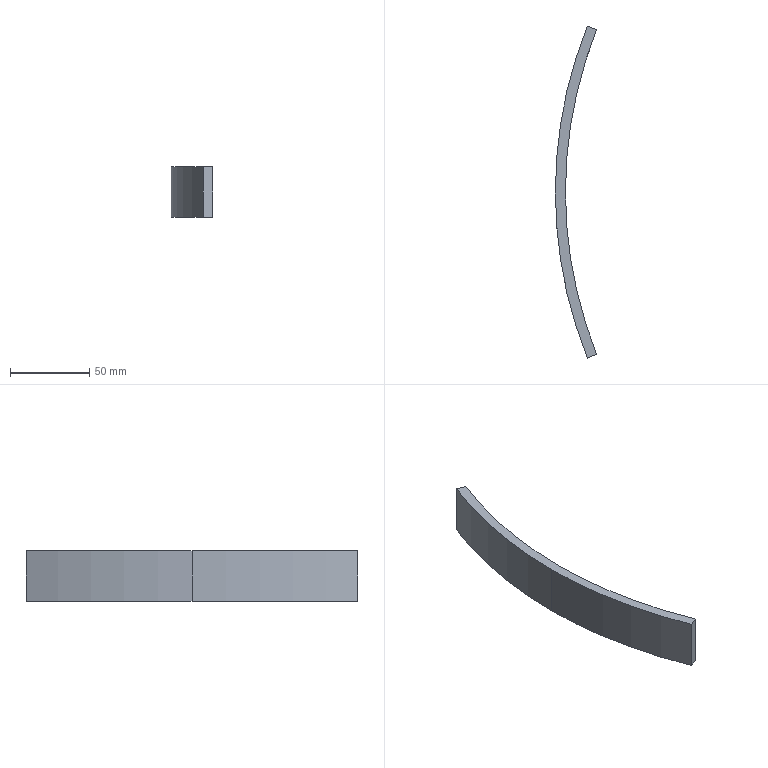Part | SolidWorks | features Extrusion 1 | 1 solid | 8 faces | box 25.986 x 209.322 x 31.75 mm | volume 42745 mm3 | cylinder 4 | plane 4 | commonest cylinder face diameters 552.7 x2 565.4 x2
STEP:
#1=CARTESIAN_POINT('',(-282.7,0.,31.75));
#2=VERTEX_POINT('',#1);
#3=CARTESIAN_POINT('',(-262.613,-104.661,31.75));
#4=VERTEX_POINT('',#3);
#5=CARTESIAN_POINT('',(0.,0.,31.75));
#6=DIRECTION('',(0.,0.,1.));
#7=DIRECTION('',(1.,0.,0.));
#8=AXIS2_PLACEMENT_3D('',#5,#6,#7);
#9=CIRCLE('',#8,282.7);
#10=EDGE_CURVE('',#2,#4,#9,.T.);
#11=ORIENTED_EDGE('',*,*,#10,.F.);
#12=CARTESIAN_POINT('',(-282.7,0.,0.));
#13=VERTEX_POINT('',#12);
#14=CARTESIAN_POINT('',(-282.7,0.,31.75));
#15=DIRECTION('',(0.,0.,-1.));
#16=VECTOR('',#15,1000.);
#17=LINE('',#14,#16);
#18=EDGE_CURVE('',#2,#13,#17,.T.);
#19=ORIENTED_EDGE('',*,*,#18,.T.);
#20=CARTESIAN_POINT('',(-262.613,-104.661,0.));
#21=VERTEX_POINT('',#20);
#22=CARTESIAN_POINT('',(0.,0.,0.));
#23=DIRECTION('',(0.,0.,1.));
#24=DIRECTION('',(1.,0.,0.));
#25=AXIS2_PLACEMENT_3D('',#22,#23,#24);
#26=CIRCLE('',#25,282.7);
#27=EDGE_CURVE('',#13,#21,#26,.T.);
#28=ORIENTED_EDGE('',*,*,#27,.T.);
#29=CARTESIAN_POINT('',(-262.613,-104.661,31.75));
#30=DIRECTION('',(0.,0.,-1.));
#31=VECTOR('',#30,1000.);
#32=LINE('',#29,#31);
#33=EDGE_CURVE('',#4,#21,#32,.T.);
#34=ORIENTED_EDGE('',*,*,#33,.F.);
#35=EDGE_LOOP('',(#11,#19,#28,#34));
#36=FACE_OUTER_BOUND('',#35,.T.);
#37=CARTESIAN_POINT('',(0.,0.,31.75));
#38=DIRECTION('',(0.,0.,-1.));
#39=DIRECTION('',(-1.,0.,0.));
#40=AXIS2_PLACEMENT_3D('',#37,#38,#39);
#41=CYLINDRICAL_SURFACE('',#40,282.7);
#42=ADVANCED_FACE('',(#36),#41,.T.);
#43=CARTESIAN_POINT('',(-276.35,0.,31.75));
#44=VERTEX_POINT('',#43);
#45=CARTESIAN_POINT('',(-256.714,102.31,31.75));
#46=VERTEX_POINT('',#45);
#47=CARTESIAN_POINT('',(0.,0.,31.75));
#48=DIRECTION('',(0.,0.,-1.));
#49=DIRECTION('',(1.,0.,0.));
#50=AXIS2_PLACEMENT_3D('',#47,#48,#49);
#51=CIRCLE('',#50,276.35);
#52=EDGE_CURVE('',#44,#46,#51,.T.);
#53=ORIENTED_EDGE('',*,*,#52,.F.);
#54=CARTESIAN_POINT('',(-276.35,0.,0.));
#55=VERTEX_POINT('',#54);
#56=CARTESIAN_POINT('',(-276.35,0.,31.75));
#57=DIRECTION('',(0.,0.,-1.));
#58=VECTOR('',#57,1000.);
#59=LINE('',#56,#58);
#60=EDGE_CURVE('',#44,#55,#59,.T.);
#61=ORIENTED_EDGE('',*,*,#60,.T.);
#62=CARTESIAN_POINT('',(-256.714,102.31,0.));
#63=VERTEX_POINT('',#62);
#64=CARTESIAN_POINT('',(0.,0.,0.));
#65=DIRECTION('',(0.,0.,-1.));
#66=DIRECTION('',(1.,0.,0.));
#67=AXIS2_PLACEMENT_3D('',#64,#65,#66);
#68=CIRCLE('',#67,276.35);
#69=EDGE_CURVE('',#55,#63,#68,.T.);
#70=ORIENTED_EDGE('',*,*,#69,.T.);
#71=CARTESIAN_POINT('',(-256.714,102.31,31.75));
#72=DIRECTION('',(0.,0.,-1.));
#73=VECTOR('',#72,1000.);
#74=LINE('',#71,#73);
#75=EDGE_CURVE('',#46,#63,#74,.T.);
#76=ORIENTED_EDGE('',*,*,#75,.F.);
#77=EDGE_LOOP('',(#53,#61,#70,#76));
#78=FACE_OUTER_BOUND('',#77,.T.);
#79=CARTESIAN_POINT('',(0.,0.,31.75));
#80=DIRECTION('',(0.,0.,-1.));
#81=DIRECTION('',(-1.,0.,0.));
#82=AXIS2_PLACEMENT_3D('',#79,#80,#81);
#83=CYLINDRICAL_SURFACE('',#82,276.35);
#84=ADVANCED_FACE('',(#78),#83,.F.);
#85=ORIENTED_EDGE('',*,*,#60,.F.);
#86=CARTESIAN_POINT('',(-256.714,-102.31,31.75));
#87=VERTEX_POINT('',#86);
#88=CARTESIAN_POINT('',(0.,0.,31.75));
#89=DIRECTION('',(0.,0.,-1.));
#90=DIRECTION('',(1.,0.,0.));
#91=AXIS2_PLACEMENT_3D('',#88,#89,#90);
#92=CIRCLE('',#91,276.35);
#93=EDGE_CURVE('',#87,#44,#92,.T.);
#94=ORIENTED_EDGE('',*,*,#93,.F.);
#95=CARTESIAN_POINT('',(-256.714,-102.31,0.));
#96=VERTEX_POINT('',#95);
#97=CARTESIAN_POINT('',(-256.714,-102.31,31.75));
#98=DIRECTION('',(0.,0.,-1.));
#99=VECTOR('',#98,1000.);
#100=LINE('',#97,#99);
#101=EDGE_CURVE('',#87,#96,#100,.T.);
#102=ORIENTED_EDGE('',*,*,#101,.T.);
#103=CARTESIAN_POINT('',(0.,0.,0.));
#104=DIRECTION('',(0.,0.,-1.));
#105=DIRECTION('',(1.,0.,0.));
#106=AXIS2_PLACEMENT_3D('',#103,#104,#105);
#107=CIRCLE('',#106,276.35);
#108=EDGE_CURVE('',#96,#55,#107,.T.);
#109=ORIENTED_EDGE('',*,*,#108,.T.);
#110=EDGE_LOOP('',(#85,#94,#102,#109));
#111=FACE_OUTER_BOUND('',#110,.T.);
#112=CARTESIAN_POINT('',(0.,0.,31.75));
#113=DIRECTION('',(0.,0.,-1.));
#114=DIRECTION('',(-1.,0.,0.));
#115=AXIS2_PLACEMENT_3D('',#112,#113,#114);
#116=CYLINDRICAL_SURFACE('',#115,276.35);
#117=ADVANCED_FACE('',(#111),#116,.F.);
#118=CARTESIAN_POINT('',(-262.613,104.661,0.));
#119=VERTEX_POINT('',#118);
#120=CARTESIAN_POINT('',(-256.714,102.31,0.));
#121=DIRECTION('',(-0.9289,0.3702,0.));
#122=VECTOR('',#121,1000.);
#123=LINE('',#120,#122);
#124=EDGE_CURVE('',#63,#119,#123,.T.);
#125=ORIENTED_EDGE('',*,*,#124,.T.);
#126=CARTESIAN_POINT('',(-262.613,104.661,31.75));
#127=VERTEX_POINT('',#126);
#128=CARTESIAN_POINT('',(-262.613,104.661,31.75));
#129=DIRECTION('',(0.,0.,-1.));
#130=VECTOR('',#129,1000.);
#131=LINE('',#128,#130);
#132=EDGE_CURVE('',#127,#119,#131,.T.);
#133=ORIENTED_EDGE('',*,*,#132,.F.);
#134=CARTESIAN_POINT('',(-256.714,102.31,31.75));
#135=DIRECTION('',(-0.9289,0.3702,0.));
#136=VECTOR('',#135,1000.);
#137=LINE('',#134,#136);
#138=EDGE_CURVE('',#46,#127,#137,.T.);
#139=ORIENTED_EDGE('',*,*,#138,.F.);
#140=ORIENTED_EDGE('',*,*,#75,.T.);
#141=EDGE_LOOP('',(#125,#133,#139,#140));
#142=FACE_OUTER_BOUND('',#141,.T.);
#143=CARTESIAN_POINT('',(-256.714,102.31,31.75));
#144=DIRECTION('',(-0.3702,-0.9289,0.));
#145=DIRECTION('',(0.9289,-0.3702,0.));
#146=AXIS2_PLACEMENT_3D('',#143,#144,#145);
#147=PLANE('',#146);
#148=ADVANCED_FACE('',(#142),#147,.F.);
#149=ORIENTED_EDGE('',*,*,#18,.F.);
#150=CARTESIAN_POINT('',(0.,0.,31.75));
#151=DIRECTION('',(0.,0.,1.));
#152=DIRECTION('',(1.,0.,0.));
#153=AXIS2_PLACEMENT_3D('',#150,#151,#152);
#154=CIRCLE('',#153,282.7);
#155=EDGE_CURVE('',#127,#2,#154,.T.);
#156=ORIENTED_EDGE('',*,*,#155,.F.);
#157=ORIENTED_EDGE('',*,*,#132,.T.);
#158=CARTESIAN_POINT('',(0.,0.,0.));
#159=DIRECTION('',(0.,0.,1.));
#160=DIRECTION('',(1.,0.,0.));
#161=AXIS2_PLACEMENT_3D('',#158,#159,#160);
#162=CIRCLE('',#161,282.7);
#163=EDGE_CURVE('',#119,#13,#162,.T.);
#164=ORIENTED_EDGE('',*,*,#163,.T.);
#165=EDGE_LOOP('',(#149,#156,#157,#164));
#166=FACE_OUTER_BOUND('',#165,.T.);
#167=CARTESIAN_POINT('',(0.,0.,31.75));
#168=DIRECTION('',(0.,0.,-1.));
#169=DIRECTION('',(-1.,0.,0.));
#170=AXIS2_PLACEMENT_3D('',#167,#168,#169);
#171=CYLINDRICAL_SURFACE('',#170,282.7);
#172=ADVANCED_FACE('',(#166),#171,.T.);
#173=CARTESIAN_POINT('',(-256.714,-102.31,0.));
#174=DIRECTION('',(0.9289,0.3702,0.));
#175=VECTOR('',#174,1000.);
#176=LINE('',#173,#175);
#177=EDGE_CURVE('',#21,#96,#176,.T.);
#178=ORIENTED_EDGE('',*,*,#177,.T.);
#179=ORIENTED_EDGE('',*,*,#101,.F.);
#180=CARTESIAN_POINT('',(-256.714,-102.31,31.75));
#181=DIRECTION('',(0.9289,0.3702,0.));
#182=VECTOR('',#181,1000.);
#183=LINE('',#180,#182);
#184=EDGE_CURVE('',#4,#87,#183,.T.);
#185=ORIENTED_EDGE('',*,*,#184,.F.);
#186=ORIENTED_EDGE('',*,*,#33,.T.);
#187=EDGE_LOOP('',(#178,#179,#185,#186));
#188=FACE_OUTER_BOUND('',#187,.T.);
#189=CARTESIAN_POINT('',(-256.714,-102.31,31.75));
#190=DIRECTION('',(-0.3702,0.9289,0.));
#191=DIRECTION('',(-0.9289,-0.3702,0.));
#192=AXIS2_PLACEMENT_3D('',#189,#190,#191);
#193=PLANE('',#192);
#194=ADVANCED_FACE('',(#188),#193,.F.);
#195=ORIENTED_EDGE('',*,*,#93,.T.);
#196=ORIENTED_EDGE('',*,*,#52,.T.);
#197=ORIENTED_EDGE('',*,*,#138,.T.);
#198=ORIENTED_EDGE('',*,*,#155,.T.);
#199=ORIENTED_EDGE('',*,*,#10,.T.);
#200=ORIENTED_EDGE('',*,*,#184,.T.);
#201=EDGE_LOOP('',(#195,#196,#197,#198,#199,#200));
#202=FACE_OUTER_BOUND('',#201,.T.);
#203=CARTESIAN_POINT('',(0.,0.,31.75));
#204=DIRECTION('',(0.,0.,1.));
#205=DIRECTION('',(1.,0.,0.));
#206=AXIS2_PLACEMENT_3D('',#203,#204,#205);
#207=PLANE('',#206);
#208=ADVANCED_FACE('',(#202),#207,.T.);
#209=ORIENTED_EDGE('',*,*,#108,.F.);
#210=ORIENTED_EDGE('',*,*,#177,.F.);
#211=ORIENTED_EDGE('',*,*,#27,.F.);
#212=ORIENTED_EDGE('',*,*,#163,.F.);
#213=ORIENTED_EDGE('',*,*,#124,.F.);
#214=ORIENTED_EDGE('',*,*,#69,.F.);
#215=EDGE_LOOP('',(#209,#210,#211,#212,#213,#214));
#216=FACE_OUTER_BOUND('',#215,.T.);
#217=CARTESIAN_POINT('',(0.,0.,0.));
#218=DIRECTION('',(0.,0.,1.));
#219=DIRECTION('',(1.,0.,0.));
#220=AXIS2_PLACEMENT_3D('',#217,#218,#219);
#221=PLANE('',#220);
#222=ADVANCED_FACE('',(#216),#221,.F.);
#223=CLOSED_SHELL('',(#42,#84,#117,#148,#172,#194,#208,#222));
#224=MANIFOLD_SOLID_BREP('',#223);
#225=CARTESIAN_POINT('',(0.,0.,0.));
#226=DIRECTION('',(0.,0.,1.));
#227=DIRECTION('',(1.,0.,0.));
#228=AXIS2_PLACEMENT_3D('',#225,#226,#227);
#229=(LENGTH_UNIT()NAMED_UNIT(*)SI_UNIT(.MILLI.,.METRE.));
#230=UNCERTAINTY_MEASURE_WITH_UNIT(LENGTH_MEASURE(0.00001),#229,'','');
#231=(NAMED_UNIT(*)PLANE_ANGLE_UNIT()SI_UNIT($,.RADIAN.));
#232=(NAMED_UNIT(*)SI_UNIT($,.STERADIAN.)SOLID_ANGLE_UNIT());
#233=(GEOMETRIC_REPRESENTATION_CONTEXT(3)GLOBAL_UNCERTAINTY_ASSIGNED_CONTEXT((#230))GLOBAL_UNIT_ASSIGNED_CONTEXT((#229,#231,#232))REPRESENTATION_CONTEXT('',''));
#234=ADVANCED_BREP_SHAPE_REPRESENTATION('',(#224,#228),#233);